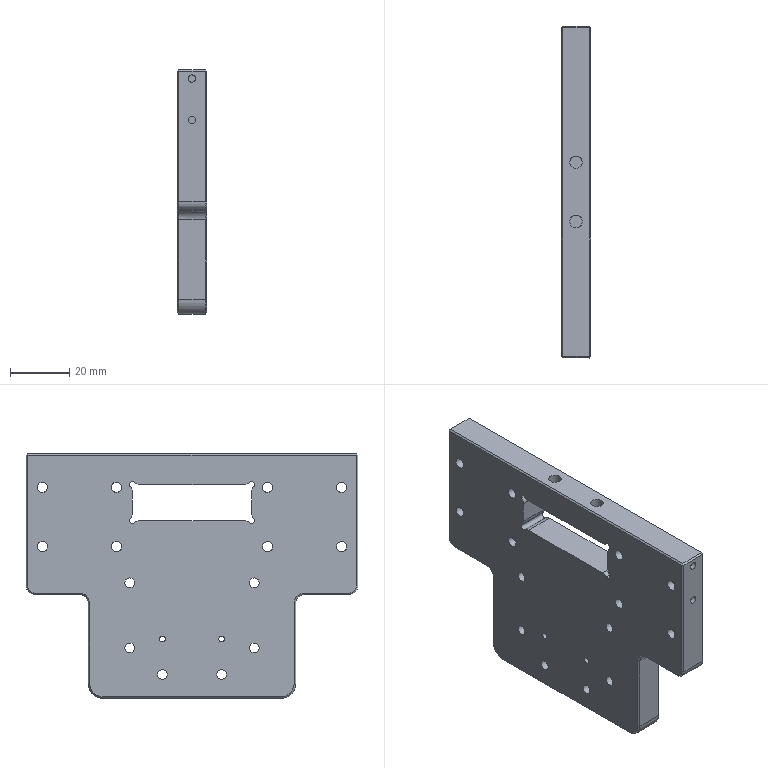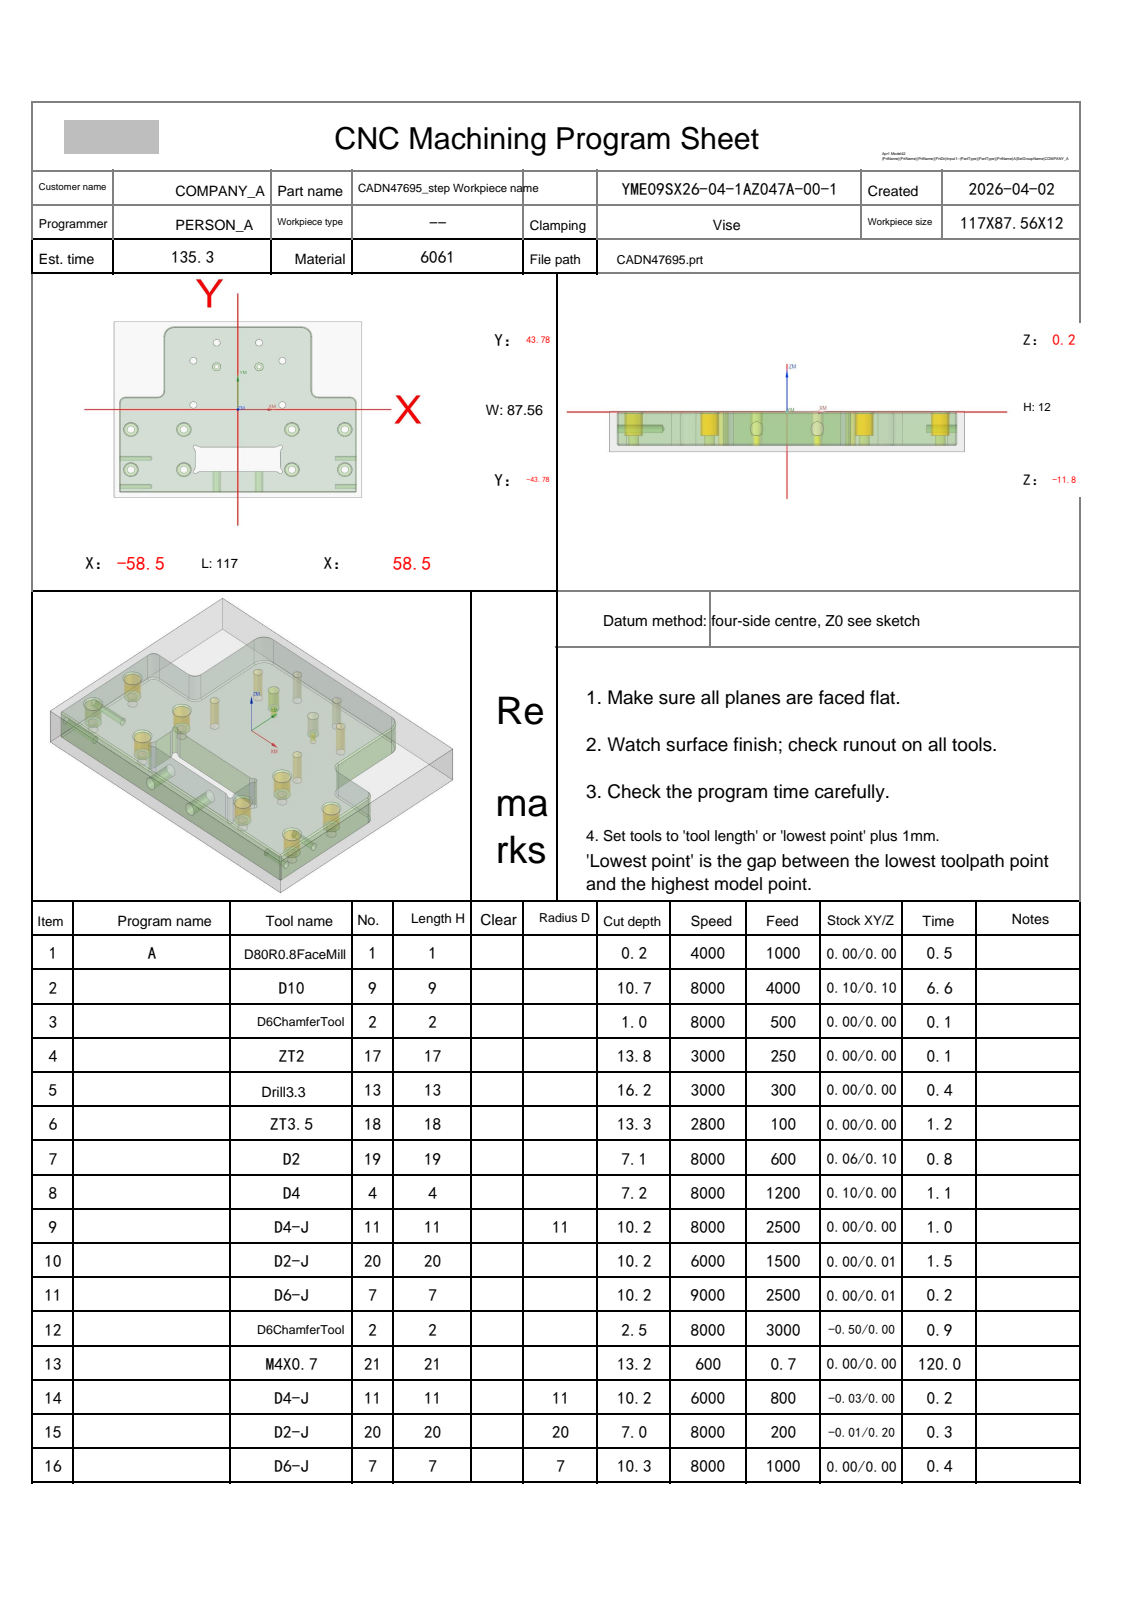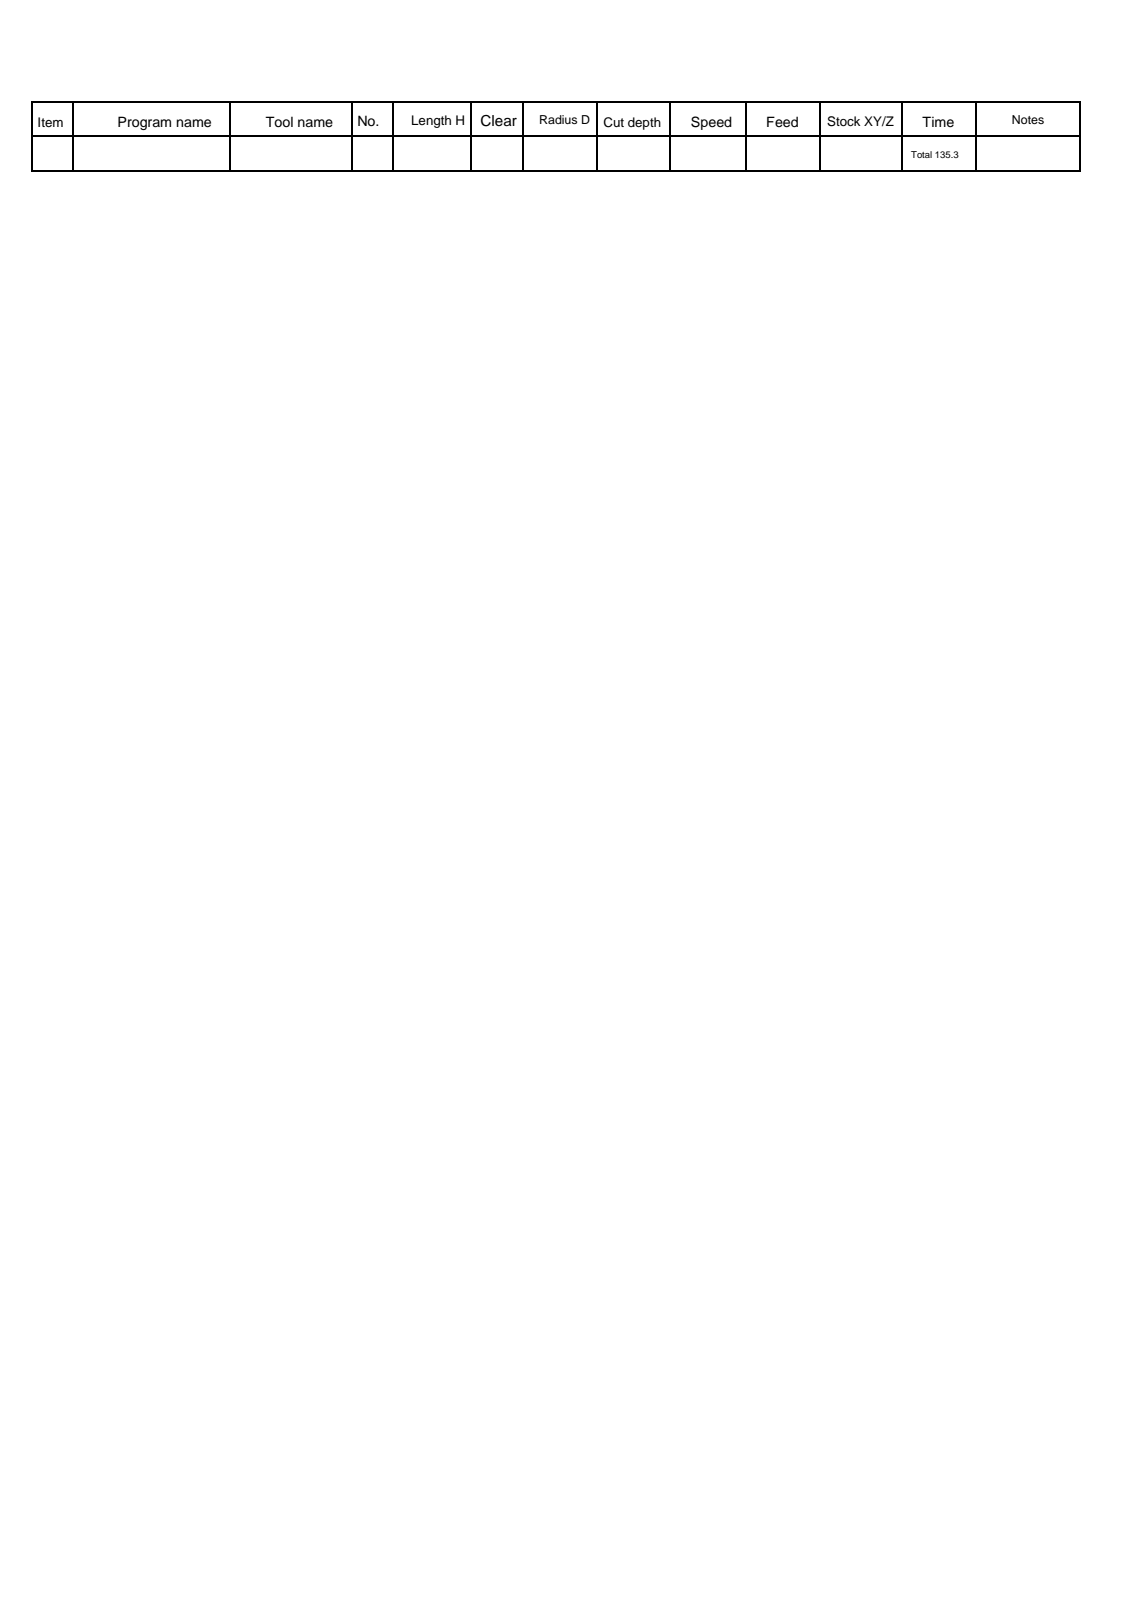NC program | NX | posted by the shop | part box 10 x 112 x 82.562 mm
Lines 2551 to 3037 of 16718:
N3 T02 M06
(D6ChamferTool  D=6. R=0. H=02 ce=0.00 di=0.10)
G00 G90 G54 X-50.5 Y-9.931 M03 S8000
G43 H02 Z20.
M08
G98 G81 X-50.5 Y-9.931 Z-.8 R1. F500.
Y-29.931
X-25.5
Y-9.931
X-21. Y2.281
X-21.002 Y24.281
X-10.003 Y33.281
X9.997
X20.998 Y24.281
Y2.281
X25.5 Y-9.931
Y-29.931
X50.5
Y-9.931
G80
G00 Z20.
G00 G90 X10.008 Y21.281 M03 S8000
Z20.
G98 G81 X10.008 Y21.281 Z-.8 R1. F500.
X-9.992
G80
G00 Z20.
G91 G28 Z0.0
M05
M09
G91 G28 Z0.0
M01
N4 T17 M06
(ZT2 D=2. DR_a=118 H=17)
G00 G90 G54 X10.008 Y21.281 M03 S3000
G43 H17 Z20.
M08
G98 G83 X10.008 Y21.281 Z-13.601 R1. F250. Q2.
X-9.992
G80
G00 Z20.
G91 G28 Z0.0
M05
M09
G91 G28 Z0.0
M01
N5 T13 M06
(Drill 3.3 D=3.3 DR_a=118 H=13)
G00 G90 G54 X-21. Y2.281 M03 S3000
G43 H13 Z20.
M08
G98 G83 X-21. Y2.281 Z-15.991 R1. F300. Q2.
X-21.002 Y24.281
X-10.003 Y33.281
X9.997
X20.998 Y24.281
Y2.281
G80
G00 Z20.
G91 G28 Z0.0
M05
M09
G91 G28 Z0.0
M01
N6 T18 M06
(ZT3.5 D=3.5 DR_a=118 H=18)
G00 G90 G54 X50.5 Y-9.931 M03 S2800
G43 H18 Z20.
M08
G98 G83 X50.5 Y-9.931 Z-13.052 R1. F100. Q2.
Y-29.931
X25.5
Y-9.931
X-25.5
Y-29.931
X-50.5
Y-9.931
G80
G00 Z20.
G91 G28 Z0.0
M05
M09
G91 G28 Z0.0
M01
N7 T19 M06
(D2  D=2. R=0. H=19 ce=0.06 di=0.10)
G00 G90 G54 X10.008 Y21.281 M03 S8000
G43 H19 Z20.
M08
Z.5
G03 X9.538 Y21.751 I-.47 J0.0 F600.
X9.068 Y21.281 I0.0 J-.47
X9.068 Y21.281 Z.3 I.94 J0.0
X9.068 Y21.281 Z.1 I.94 J0.0
X9.068 Y21.281 Z-.1 I.94 J0.0
X9.068 Y21.281 Z-.3 I.94 J0.0
X9.068 Y21.281 Z-.5 I.94 J0.0
X9.068 Y21.281 Z-.7 I.94 J0.0
X9.068 Y21.281 Z-.9 I.94 J0.0
X9.068 Y21.281 Z-1.1 I.94 J0.0
X9.068 Y21.281 Z-1.3 I.94 J0.0
X9.068 Y21.281 Z-1.5 I.94 J0.0
X9.068 Y21.281 Z-1.7 I.94 J0.0
X9.068 Y21.281 Z-1.9 I.94 J0.0
X9.068 Y21.281 Z-2.1 I.94 J0.0
X9.068 Y21.281 Z-2.3 I.94 J0.0
X9.068 Y21.281 Z-2.5 I.94 J0.0
X9.068 Y21.281 Z-2.7 I.94 J0.0
X9.068 Y21.281 Z-2.9 I.94 J0.0
X9.068 Y21.281 Z-3.1 I.94 J0.0
X9.068 Y21.281 Z-3.3 I.94 J0.0
X9.068 Y21.281 Z-3.5 I.94 J0.0
X9.068 Y21.281 Z-3.7 I.94 J0.0
X9.068 Y21.281 Z-3.9 I.94 J0.0
X9.068 Y21.281 Z-4.1 I.94 J0.0
X9.068 Y21.281 Z-4.3 I.94 J0.0
X9.068 Y21.281 Z-4.5 I.94 J0.0
X9.068 Y21.281 Z-4.7 I.94 J0.0
X9.068 Y21.281 Z-4.9 I.94 J0.0
X9.068 Y21.281 Z-5.1 I.94 J0.0
X9.068 Y21.281 Z-5.3 I.94 J0.0
X9.068 Y21.281 Z-5.5 I.94 J0.0
X9.068 Y21.281 Z-5.7 I.94 J0.0
X9.068 Y21.281 Z-5.9 I.94 J0.0
X9.068 Y21.281 Z-6.1 I.94 J0.0
X9.068 Y21.281 Z-6.3 I.94 J0.0
X9.068 Y21.281 Z-6.5 I.94 J0.0
X9.068 Y21.281 Z-6.7 I.94 J0.0
X9.068 Y21.281 Z-6.9 I.94 J0.0
X10.008 Y20.341 I.94 J0.0
X10.948 Y21.281 I0.0 J.94
X10.008 Y22.221 I-.94 J0.0
X9.068 Y21.281 I0.0 J-.94
X9.538 Y20.811 I.47 J0.0
X10.008 Y21.281 I0.0 J.47
G00 Z20.
G00 G90 X-9.992 Y21.281 M03 S8000
Z20.
Z.5
G03 X-10.462 Y21.751 I-.47 J0.0 F600.
X-10.932 Y21.281 I0.0 J-.47
X-10.932 Y21.281 Z.3 I.94 J0.0
X-10.932 Y21.281 Z.1 I.94 J0.0
X-10.932 Y21.281 Z-.1 I.94 J0.0
X-10.932 Y21.281 Z-.3 I.94 J0.0
X-10.932 Y21.281 Z-.5 I.94 J0.0
X-10.932 Y21.281 Z-.7 I.94 J0.0
X-10.932 Y21.281 Z-.9 I.94 J0.0
X-10.932 Y21.281 Z-1.1 I.94 J0.0
X-10.932 Y21.281 Z-1.3 I.94 J0.0
X-10.932 Y21.281 Z-1.5 I.94 J0.0
X-10.932 Y21.281 Z-1.7 I.94 J0.0
X-10.932 Y21.281 Z-1.9 I.94 J0.0
X-10.932 Y21.281 Z-2.1 I.94 J0.0
X-10.932 Y21.281 Z-2.3 I.94 J0.0
X-10.932 Y21.281 Z-2.5 I.94 J0.0
X-10.932 Y21.281 Z-2.7 I.94 J0.0
X-10.932 Y21.281 Z-2.9 I.94 J0.0
X-10.932 Y21.281 Z-3.1 I.94 J0.0
X-10.932 Y21.281 Z-3.3 I.94 J0.0
X-10.932 Y21.281 Z-3.5 I.94 J0.0
X-10.932 Y21.281 Z-3.7 I.94 J0.0
X-10.932 Y21.281 Z-3.9 I.94 J0.0
X-10.932 Y21.281 Z-4.1 I.94 J0.0
X-10.932 Y21.281 Z-4.3 I.94 J0.0
X-10.932 Y21.281 Z-4.5 I.94 J0.0
X-10.932 Y21.281 Z-4.7 I.94 J0.0
X-10.932 Y21.281 Z-4.9 I.94 J0.0
X-10.932 Y21.281 Z-5.1 I.94 J0.0
X-10.932 Y21.281 Z-5.3 I.94 J0.0
X-10.932 Y21.281 Z-5.5 I.94 J0.0
X-10.932 Y21.281 Z-5.7 I.94 J0.0
X-10.932 Y21.281 Z-5.9 I.94 J0.0
X-10.932 Y21.281 Z-6.1 I.94 J0.0
X-10.932 Y21.281 Z-6.3 I.94 J0.0
X-10.932 Y21.281 Z-6.5 I.94 J0.0
X-10.932 Y21.281 Z-6.7 I.94 J0.0
X-10.932 Y21.281 Z-6.9 I.94 J0.0
X-9.992 Y20.341 I.94 J0.0
X-9.052 Y21.281 I0.0 J.94
X-9.992 Y22.221 I-.94 J0.0
X-10.932 Y21.281 I0.0 J-.94
X-10.462 Y20.811 I.47 J0.0
X-9.992 Y21.281 I0.0 J.47
G00 Z20.
G91 G28 Z0.0
M05
M09
G91 G28 Z0.0
M01
N8 T04 M06
(D4  D=4. R=0. H=04 ce=0.10 di=0.00)
G00 G90 G54 X-50.5 Y-29.931 M03 S8000
G43 H04 Z20.
M08
Z.5
G03 X-50.95 Y-29.481 I-.45 J0.0 F1200.
X-51.4 Y-29.931 I0.0 J-.45
X-51.4 Y-29.931 Z.2 I.9 J0.0
X-51.4 Y-29.931 Z-.1 I.9 J0.0
X-51.4 Y-29.931 Z-.4 I.9 J0.0
X-51.4 Y-29.931 Z-.7 I.9 J0.0
X-51.4 Y-29.931 Z-1. I.9 J0.0
X-51.4 Y-29.931 Z-1.3 I.9 J0.0
X-51.4 Y-29.931 Z-1.6 I.9 J0.0
X-51.4 Y-29.931 Z-1.9 I.9 J0.0
X-51.4 Y-29.931 Z-2.2 I.9 J0.0
X-51.4 Y-29.931 Z-2.5 I.9 J0.0
X-51.4 Y-29.931 Z-2.8 I.9 J0.0
X-51.4 Y-29.931 Z-3.1 I.9 J0.0
X-51.4 Y-29.931 Z-3.4 I.9 J0.0
X-51.4 Y-29.931 Z-3.7 I.9 J0.0
X-51.4 Y-29.931 Z-4. I.9 J0.0
X-51.4 Y-29.931 Z-4.3 I.9 J0.0
X-51.4 Y-29.931 Z-4.6 I.9 J0.0
X-51.4 Y-29.931 Z-4.9 I.9 J0.0
X-51.4 Y-29.931 Z-5.2 I.9 J0.0
X-51.4 Y-29.931 Z-5.5 I.9 J0.0
X-51.4 Y-29.931 Z-5.8 I.9 J0.0
X-51.4 Y-29.931 Z-6.1 I.9 J0.0
X-51.4 Y-29.931 Z-6.4 I.9 J0.0
X-51.4 Y-29.931 Z-6.7 I.9 J0.0
X-51.4 Y-29.931 Z-7. I.9 J0.0
X-50.5 Y-30.831 I.9 J0.0
X-49.6 Y-29.931 I0.0 J.9
X-50.5 Y-29.031 I-.9 J0.0
X-51.4 Y-29.931 I0.0 J-.9
X-50.95 Y-30.381 I.45 J0.0
X-50.5 Y-29.931 I0.0 J.45
G00 Z20.
Y-9.931
Z.5
G03 X-50.95 Y-9.481 I-.45 J0.0
X-51.4 Y-9.931 I0.0 J-.45
X-51.4 Y-9.931 Z.2 I.9 J0.0
X-51.4 Y-9.931 Z-.1 I.9 J0.0
X-51.4 Y-9.931 Z-.4 I.9 J0.0
X-51.4 Y-9.931 Z-.7 I.9 J0.0
X-51.4 Y-9.931 Z-1. I.9 J0.0
X-51.4 Y-9.931 Z-1.3 I.9 J0.0
X-51.4 Y-9.931 Z-1.6 I.9 J0.0
X-51.4 Y-9.931 Z-1.9 I.9 J0.0
X-51.4 Y-9.931 Z-2.2 I.9 J0.0
X-51.4 Y-9.931 Z-2.5 I.9 J0.0
X-51.4 Y-9.931 Z-2.8 I.9 J0.0
X-51.4 Y-9.931 Z-3.1 I.9 J0.0
X-51.4 Y-9.931 Z-3.4 I.9 J0.0
X-51.4 Y-9.931 Z-3.7 I.9 J0.0
X-51.4 Y-9.931 Z-4. I.9 J0.0
X-51.4 Y-9.931 Z-4.3 I.9 J0.0
X-51.4 Y-9.931 Z-4.6 I.9 J0.0
X-51.4 Y-9.931 Z-4.9 I.9 J0.0
X-51.4 Y-9.931 Z-5.2 I.9 J0.0
X-51.4 Y-9.931 Z-5.5 I.9 J0.0
X-51.4 Y-9.931 Z-5.8 I.9 J0.0
X-51.4 Y-9.931 Z-6.1 I.9 J0.0
X-51.4 Y-9.931 Z-6.4 I.9 J0.0
X-51.4 Y-9.931 Z-6.7 I.9 J0.0
X-51.4 Y-9.931 Z-7. I.9 J0.0
X-50.5 Y-10.831 I.9 J0.0
X-49.6 Y-9.931 I0.0 J.9
X-50.5 Y-9.031 I-.9 J0.0
X-51.4 Y-9.931 I0.0 J-.9
X-50.95 Y-10.381 I.45 J0.0
X-50.5 Y-9.931 I0.0 J.45
G00 Z20.
X-25.5
Z.5
G03 X-25.95 Y-9.481 I-.45 J0.0
X-26.4 Y-9.931 I0.0 J-.45
X-26.4 Y-9.931 Z.2 I.9 J0.0
X-26.4 Y-9.931 Z-.1 I.9 J0.0
X-26.4 Y-9.931 Z-.4 I.9 J0.0
X-26.4 Y-9.931 Z-.7 I.9 J0.0
X-26.4 Y-9.931 Z-1. I.9 J0.0
X-26.4 Y-9.931 Z-1.3 I.9 J0.0
X-26.4 Y-9.931 Z-1.6 I.9 J0.0
X-26.4 Y-9.931 Z-1.9 I.9 J0.0
X-26.4 Y-9.931 Z-2.2 I.9 J0.0
X-26.4 Y-9.931 Z-2.5 I.9 J0.0
X-26.4 Y-9.931 Z-2.8 I.9 J0.0
X-26.4 Y-9.931 Z-3.1 I.9 J0.0
X-26.4 Y-9.931 Z-3.4 I.9 J0.0
X-26.4 Y-9.931 Z-3.7 I.9 J0.0
X-26.4 Y-9.931 Z-4. I.9 J0.0
X-26.4 Y-9.931 Z-4.3 I.9 J0.0
X-26.4 Y-9.931 Z-4.6 I.9 J0.0
X-26.4 Y-9.931 Z-4.9 I.9 J0.0
X-26.4 Y-9.931 Z-5.2 I.9 J0.0
X-26.4 Y-9.931 Z-5.5 I.9 J0.0
X-26.4 Y-9.931 Z-5.8 I.9 J0.0
X-26.4 Y-9.931 Z-6.1 I.9 J0.0
X-26.4 Y-9.931 Z-6.4 I.9 J0.0
X-26.4 Y-9.931 Z-6.7 I.9 J0.0
X-26.4 Y-9.931 Z-7. I.9 J0.0
X-25.5 Y-10.831 I.9 J0.0
X-24.6 Y-9.931 I0.0 J.9
X-25.5 Y-9.031 I-.9 J0.0
X-26.4 Y-9.931 I0.0 J-.9
X-25.95 Y-10.381 I.45 J0.0
X-25.5 Y-9.931 I0.0 J.45
G00 Z20.
Y-29.931
Z.5
G03 X-25.95 Y-29.481 I-.45 J0.0
X-26.4 Y-29.931 I0.0 J-.45
X-26.4 Y-29.931 Z.2 I.9 J0.0
X-26.4 Y-29.931 Z-.1 I.9 J0.0
X-26.4 Y-29.931 Z-.4 I.9 J0.0
X-26.4 Y-29.931 Z-.7 I.9 J0.0
X-26.4 Y-29.931 Z-1. I.9 J0.0
X-26.4 Y-29.931 Z-1.3 I.9 J0.0
X-26.4 Y-29.931 Z-1.6 I.9 J0.0
X-26.4 Y-29.931 Z-1.9 I.9 J0.0
X-26.4 Y-29.931 Z-2.2 I.9 J0.0
X-26.4 Y-29.931 Z-2.5 I.9 J0.0
X-26.4 Y-29.931 Z-2.8 I.9 J0.0
X-26.4 Y-29.931 Z-3.1 I.9 J0.0
X-26.4 Y-29.931 Z-3.4 I.9 J0.0
X-26.4 Y-29.931 Z-3.7 I.9 J0.0
X-26.4 Y-29.931 Z-4. I.9 J0.0
X-26.4 Y-29.931 Z-4.3 I.9 J0.0
X-26.4 Y-29.931 Z-4.6 I.9 J0.0
X-26.4 Y-29.931 Z-4.9 I.9 J0.0
X-26.4 Y-29.931 Z-5.2 I.9 J0.0
X-26.4 Y-29.931 Z-5.5 I.9 J0.0
X-26.4 Y-29.931 Z-5.8 I.9 J0.0
X-26.4 Y-29.931 Z-6.1 I.9 J0.0
X-26.4 Y-29.931 Z-6.4 I.9 J0.0
X-26.4 Y-29.931 Z-6.7 I.9 J0.0
X-26.4 Y-29.931 Z-7. I.9 J0.0
X-25.5 Y-30.831 I.9 J0.0
X-24.6 Y-29.931 I0.0 J.9
X-25.5 Y-29.031 I-.9 J0.0
X-26.4 Y-29.931 I0.0 J-.9
X-25.95 Y-30.381 I.45 J0.0
X-25.5 Y-29.931 I0.0 J.45
G00 Z20.
X25.5
Z.5
G03 X25.05 Y-29.481 I-.45 J0.0
X24.6 Y-29.931 I0.0 J-.45
X24.6 Y-29.931 Z.2 I.9 J0.0
X24.6 Y-29.931 Z-.1 I.9 J0.0
X24.6 Y-29.931 Z-.4 I.9 J0.0
X24.6 Y-29.931 Z-.7 I.9 J0.0
X24.6 Y-29.931 Z-1. I.9 J0.0
X24.6 Y-29.931 Z-1.3 I.9 J0.0
X24.6 Y-29.931 Z-1.6 I.9 J0.0
X24.6 Y-29.931 Z-1.9 I.9 J0.0
X24.6 Y-29.931 Z-2.2 I.9 J0.0
X24.6 Y-29.931 Z-2.5 I.9 J0.0
X24.6 Y-29.931 Z-2.8 I.9 J0.0
X24.6 Y-29.931 Z-3.1 I.9 J0.0
X24.6 Y-29.931 Z-3.4 I.9 J0.0
X24.6 Y-29.931 Z-3.7 I.9 J0.0
X24.6 Y-29.931 Z-4. I.9 J0.0
X24.6 Y-29.931 Z-4.3 I.9 J0.0
X24.6 Y-29.931 Z-4.6 I.9 J0.0
X24.6 Y-29.931 Z-4.9 I.9 J0.0
X24.6 Y-29.931 Z-5.2 I.9 J0.0
X24.6 Y-29.931 Z-5.5 I.9 J0.0
X24.6 Y-29.931 Z-5.8 I.9 J0.0
X24.6 Y-29.931 Z-6.1 I.9 J0.0
X24.6 Y-29.931 Z-6.4 I.9 J0.0
X24.6 Y-29.931 Z-6.7 I.9 J0.0
X24.6 Y-29.931 Z-7. I.9 J0.0
X25.5 Y-30.831 I.9 J0.0
X26.4 Y-29.931 I0.0 J.9
X25.5 Y-29.031 I-.9 J0.0
X24.6 Y-29.931 I0.0 J-.9
X25.05 Y-30.381 I.45 J0.0
X25.5 Y-29.931 I0.0 J.45
G00 Z20.
Y-9.931
Z.5
G03 X25.05 Y-9.481 I-.45 J0.0
X24.6 Y-9.931 I0.0 J-.45
X24.6 Y-9.931 Z.2 I.9 J0.0
X24.6 Y-9.931 Z-.1 I.9 J0.0
X24.6 Y-9.931 Z-.4 I.9 J0.0
X24.6 Y-9.931 Z-.7 I.9 J0.0
X24.6 Y-9.931 Z-1. I.9 J0.0
X24.6 Y-9.931 Z-1.3 I.9 J0.0
X24.6 Y-9.931 Z-1.6 I.9 J0.0
X24.6 Y-9.931 Z-1.9 I.9 J0.0
X24.6 Y-9.931 Z-2.2 I.9 J0.0
X24.6 Y-9.931 Z-2.5 I.9 J0.0
X24.6 Y-9.931 Z-2.8 I.9 J0.0
X24.6 Y-9.931 Z-3.1 I.9 J0.0
X24.6 Y-9.931 Z-3.4 I.9 J0.0
X24.6 Y-9.931 Z-3.7 I.9 J0.0
X24.6 Y-9.931 Z-4. I.9 J0.0
X24.6 Y-9.931 Z-4.3 I.9 J0.0
X24.6 Y-9.931 Z-4.6 I.9 J0.0
X24.6 Y-9.931 Z-4.9 I.9 J0.0
X24.6 Y-9.931 Z-5.2 I.9 J0.0
X24.6 Y-9.931 Z-5.5 I.9 J0.0
X24.6 Y-9.931 Z-5.8 I.9 J0.0
X24.6 Y-9.931 Z-6.1 I.9 J0.0
X24.6 Y-9.931 Z-6.4 I.9 J0.0
X24.6 Y-9.931 Z-6.7 I.9 J0.0
X24.6 Y-9.931 Z-7. I.9 J0.0
X25.5 Y-10.831 I.9 J0.0
X26.4 Y-9.931 I0.0 J.9
X25.5 Y-9.031 I-.9 J0.0
X24.6 Y-9.931 I0.0 J-.9
X25.05 Y-10.381 I.45 J0.0
X25.5 Y-9.931 I0.0 J.45
G00 Z20.
X50.5
Z.5
G03 X50.05 Y-9.481 I-.45 J0.0
X49.6 Y-9.931 I0.0 J-.45
X49.6 Y-9.931 Z.2 I.9 J0.0
X49.6 Y-9.931 Z-.1 I.9 J0.0
X49.6 Y-9.931 Z-.4 I.9 J0.0
X49.6 Y-9.931 Z-.7 I.9 J0.0
X49.6 Y-9.931 Z-1. I.9 J0.0
X49.6 Y-9.931 Z-1.3 I.9 J0.0
X49.6 Y-9.931 Z-1.6 I.9 J0.0
X49.6 Y-9.931 Z-1.9 I.9 J0.0
X49.6 Y-9.931 Z-2.2 I.9 J0.0
X49.6 Y-9.931 Z-2.5 I.9 J0.0
X49.6 Y-9.931 Z-2.8 I.9 J0.0
X49.6 Y-9.931 Z-3.1 I.9 J0.0
X49.6 Y-9.931 Z-3.4 I.9 J0.0
X49.6 Y-9.931 Z-3.7 I.9 J0.0
X49.6 Y-9.931 Z-4. I.9 J0.0
X49.6 Y-9.931 Z-4.3 I.9 J0.0
X49.6 Y-9.931 Z-4.6 I.9 J0.0
X49.6 Y-9.931 Z-4.9 I.9 J0.0
X49.6 Y-9.931 Z-5.2 I.9 J0.0
X49.6 Y-9.931 Z-5.5 I.9 J0.0
X49.6 Y-9.931 Z-5.8 I.9 J0.0
X49.6 Y-9.931 Z-6.1 I.9 J0.0
X49.6 Y-9.931 Z-6.4 I.9 J0.0
X49.6 Y-9.931 Z-6.7 I.9 J0.0
X49.6 Y-9.931 Z-7. I.9 J0.0
X50.5 Y-10.831 I.9 J0.0
X51.4 Y-9.931 I0.0 J.9
X50.5 Y-9.031 I-.9 J0.0
X49.6 Y-9.931 I0.0 J-.9
X50.05 Y-10.381 I.45 J0.0
X50.5 Y-9.931 I0.0 J.45
G00 Z20.
Y-29.931
Z.5
G03 X50.05 Y-29.481 I-.45 J0.0
X49.6 Y-29.931 I0.0 J-.45
X49.6 Y-29.931 Z.2 I.9 J0.0
X49.6 Y-29.931 Z-.1 I.9 J0.0
X49.6 Y-29.931 Z-.4 I.9 J0.0
X49.6 Y-29.931 Z-.7 I.9 J0.0
X49.6 Y-29.931 Z-1. I.9 J0.0
X49.6 Y-29.931 Z-1.3 I.9 J0.0
X49.6 Y-29.931 Z-1.6 I.9 J0.0
X49.6 Y-29.931 Z-1.9 I.9 J0.0
X49.6 Y-29.931 Z-2.2 I.9 J0.0
X49.6 Y-29.931 Z-2.5 I.9 J0.0
X49.6 Y-29.931 Z-2.8 I.9 J0.0
X49.6 Y-29.931 Z-3.1 I.9 J0.0
X49.6 Y-29.931 Z-3.4 I.9 J0.0
X49.6 Y-29.931 Z-3.7 I.9 J0.0
X49.6 Y-29.931 Z-4. I.9 J0.0
X49.6 Y-29.931 Z-4.3 I.9 J0.0
X49.6 Y-29.931 Z-4.6 I.9 J0.0
X49.6 Y-29.931 Z-4.9 I.9 J0.0
X49.6 Y-29.931 Z-5.2 I.9 J0.0
X49.6 Y-29.931 Z-5.5 I.9 J0.0
X49.6 Y-29.931 Z-5.8 I.9 J0.0
X49.6 Y-29.931 Z-6.1 I.9 J0.0
X49.6 Y-29.931 Z-6.4 I.9 J0.0
X49.6 Y-29.931 Z-6.7 I.9 J0.0
X49.6 Y-29.931 Z-7. I.9 J0.0
X50.5 Y-30.831 I.9 J0.0
X51.4 Y-29.931 I0.0 J.9
X50.5 Y-29.031 I-.9 J0.0
X49.6 Y-29.931 I0.0 J-.9
X50.05 Y-30.381 I.45 J0.0
X50.5 Y-29.931 I0.0 J.45
G00 Z20.
G91 G28 Z0.0
M05
M09
G91 G28 Z0.0
M01